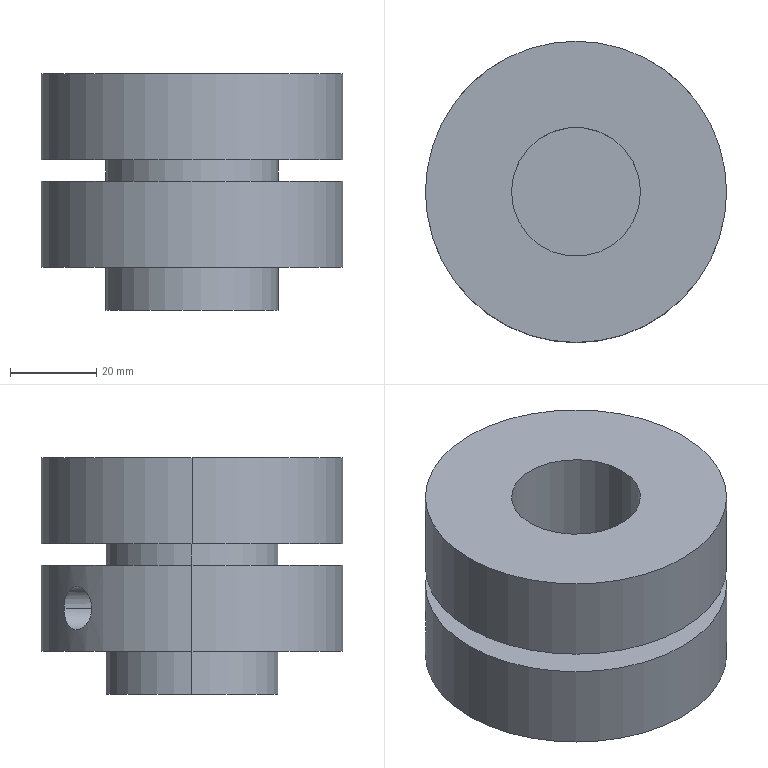Part | SolidWorks | features ICE 3, RevCut 2, Extrusion 1 | 1 solid | 22 faces | box 70 x 70 x 55 mm | volume 152574 mm3 | cylinder 14 | plane 8 | commonest cylinder face diameters 10 x4 40 x4 70 x4 30 x2
STEP:
#1=CARTESIAN_POINT('',(18.437,29.75,-15.));
#2=VERTEX_POINT('',#1);
#3=CARTESIAN_POINT('',(26.097,23.323,-15.));
#4=VERTEX_POINT('',#3);
#5=CARTESIAN_POINT('',(18.437,29.75,-15.));
#6=CARTESIAN_POINT('',(18.437,29.75,-15.326));
#7=CARTESIAN_POINT('',(18.464,29.734,-15.651));
#8=CARTESIAN_POINT('',(18.574,29.665,-16.297));
#9=CARTESIAN_POINT('',(18.656,29.614,-16.612));
#10=CARTESIAN_POINT('',(18.868,29.479,-17.214));
#11=CARTESIAN_POINT('',(19.,29.394,-17.505));
#12=CARTESIAN_POINT('',(19.308,29.193,-18.051));
#13=CARTESIAN_POINT('',(19.481,29.078,-18.303));
#14=CARTESIAN_POINT('',(19.864,28.818,-18.764));
#15=CARTESIAN_POINT('',(20.076,28.671,-18.975));
#16=CARTESIAN_POINT('',(20.519,28.356,-19.338));
#17=CARTESIAN_POINT('',(20.751,28.186,-19.491));
#18=CARTESIAN_POINT('',(21.115,27.914,-19.68));
#19=CARTESIAN_POINT('',(21.24,27.819,-19.736));
#20=CARTESIAN_POINT('',(21.489,27.627,-19.832));
#21=CARTESIAN_POINT('',(21.613,27.53,-19.871));
#22=CARTESIAN_POINT('',(21.989,27.232,-19.967));
#23=CARTESIAN_POINT('',(22.242,27.026,-20.));
#24=CARTESIAN_POINT('',(22.748,26.601,-20.));
#25=CARTESIAN_POINT('',(22.994,26.389,-19.968));
#26=CARTESIAN_POINT('',(23.473,25.964,-19.841));
#27=CARTESIAN_POINT('',(23.708,25.749,-19.745));
#28=CARTESIAN_POINT('',(24.15,25.335,-19.494));
#29=CARTESIAN_POINT('',(24.358,25.135,-19.341));
#30=CARTESIAN_POINT('',(24.746,24.753,-18.979));
#31=CARTESIAN_POINT('',(24.928,24.57,-18.768));
#32=CARTESIAN_POINT('',(25.251,24.238,-18.308));
#33=CARTESIAN_POINT('',(25.394,24.087,-18.057));
#34=CARTESIAN_POINT('',(25.647,23.818,-17.51));
#35=CARTESIAN_POINT('',(25.753,23.703,-17.22));
#36=CARTESIAN_POINT('',(25.923,23.517,-16.619));
#37=CARTESIAN_POINT('',(25.988,23.444,-16.304));
#38=CARTESIAN_POINT('',(26.075,23.347,-15.658));
#39=CARTESIAN_POINT('',(26.097,23.323,-15.331));
#40=CARTESIAN_POINT('',(26.097,23.323,-15.));
#41=B_SPLINE_CURVE_WITH_KNOTS('',3,(#5,#6,#7,#8,#9,#10,#11,#12,#13,#14,#15,#16,#17,#18,#19,#20,#21,#22,#23,#24,#25,#26,#27,#28,#29,#30,#31,#32,#33,#34,#35,#36,#37,#38,#39,#40),.UNSPECIFIED.,.F.,.F.,(4,2,2,2,2,2,2,2,2,2,2,2,2,2,2,2,2,4),(0.01565,0.01663,0.01761,0.01859,0.01956,0.02054,0.02152,0.02201,0.0225,0.02348,0.02445,0.02543,0.02641,0.02739,0.02837,0.02934,0.03032,0.0313),.UNSPECIFIED.);
#42=EDGE_CURVE('',#2,#4,#41,.T.);
#43=ORIENTED_EDGE('',*,*,#42,.F.);
#44=CARTESIAN_POINT('',(8.621,18.052,-15.));
#45=VERTEX_POINT('',#44);
#46=CARTESIAN_POINT('',(8.621,18.052,-15.));
#47=DIRECTION('',(-0.6428,-0.766,0.));
#48=VECTOR('',#47,1000.);
#49=LINE('',#46,#48);
#50=EDGE_CURVE('',#2,#45,#49,.T.);
#51=ORIENTED_EDGE('',*,*,#50,.T.);
#52=CARTESIAN_POINT('',(16.281,11.624,-15.));
#53=VERTEX_POINT('',#52);
#54=CARTESIAN_POINT('',(12.451,14.838,-15.));
#55=DIRECTION('',(-0.6428,-0.766,0.));
#56=DIRECTION('',(0.766,-0.6428,0.));
#57=AXIS2_PLACEMENT_3D('',#54,#55,#56);
#58=CIRCLE('',#57,5.);
#59=EDGE_CURVE('',#45,#53,#58,.T.);
#60=ORIENTED_EDGE('',*,*,#59,.T.);
#61=CARTESIAN_POINT('',(16.281,11.624,-15.));
#62=DIRECTION('',(-0.6428,-0.766,0.));
#63=VECTOR('',#62,1000.);
#64=LINE('',#61,#63);
#65=EDGE_CURVE('',#4,#53,#64,.T.);
#66=ORIENTED_EDGE('',*,*,#65,.F.);
#67=EDGE_LOOP('',(#43,#51,#60,#66));
#68=FACE_OUTER_BOUND('',#67,.T.);
#69=CARTESIAN_POINT('',(12.451,14.838,-15.));
#70=DIRECTION('',(-0.6428,-0.766,0.));
#71=DIRECTION('',(0.766,-0.6428,0.));
#72=AXIS2_PLACEMENT_3D('',#69,#70,#71);
#73=CYLINDRICAL_SURFACE('',#72,5.);
#74=ADVANCED_FACE('',(#68),#73,.F.);
#75=CARTESIAN_POINT('',(-26.097,23.323,-15.));
#76=VERTEX_POINT('',#75);
#77=CARTESIAN_POINT('',(-18.437,29.75,-15.));
#78=VERTEX_POINT('',#77);
#79=CARTESIAN_POINT('',(-26.097,23.323,-15.));
#80=CARTESIAN_POINT('',(-26.097,23.323,-15.326));
#81=CARTESIAN_POINT('',(-26.076,23.347,-15.651));
#82=CARTESIAN_POINT('',(-25.989,23.443,-16.297));
#83=CARTESIAN_POINT('',(-25.924,23.515,-16.612));
#84=CARTESIAN_POINT('',(-25.755,23.7,-17.214));
#85=CARTESIAN_POINT('',(-25.649,23.816,-17.505));
#86=CARTESIAN_POINT('',(-25.397,24.084,-18.051));
#87=CARTESIAN_POINT('',(-25.254,24.234,-18.303));
#88=CARTESIAN_POINT('',(-24.931,24.566,-18.764));
#89=CARTESIAN_POINT('',(-24.75,24.749,-18.975));
#90=CARTESIAN_POINT('',(-24.362,25.131,-19.338));
#91=CARTESIAN_POINT('',(-24.155,25.331,-19.491));
#92=CARTESIAN_POINT('',(-23.823,25.642,-19.68));
#93=CARTESIAN_POINT('',(-23.708,25.748,-19.736));
#94=CARTESIAN_POINT('',(-23.476,25.959,-19.832));
#95=CARTESIAN_POINT('',(-23.358,26.066,-19.871));
#96=CARTESIAN_POINT('',(-23.,26.384,-19.967));
#97=CARTESIAN_POINT('',(-22.753,26.597,-20.));
#98=CARTESIAN_POINT('',(-22.247,27.022,-20.));
#99=CARTESIAN_POINT('',(-21.995,27.227,-19.968));
#100=CARTESIAN_POINT('',(-21.493,27.625,-19.841));
#101=CARTESIAN_POINT('',(-21.241,27.819,-19.745));
#102=CARTESIAN_POINT('',(-20.756,28.183,-19.494));
#103=CARTESIAN_POINT('',(-20.524,28.352,-19.341));
#104=CARTESIAN_POINT('',(-20.08,28.669,-18.979));
#105=CARTESIAN_POINT('',(-19.868,28.815,-18.768));
#106=CARTESIAN_POINT('',(-19.485,29.076,-18.308));
#107=CARTESIAN_POINT('',(-19.311,29.191,-18.057));
#108=CARTESIAN_POINT('',(-19.002,29.393,-17.51));
#109=CARTESIAN_POINT('',(-18.871,29.477,-17.22));
#110=CARTESIAN_POINT('',(-18.658,29.612,-16.619));
#111=CARTESIAN_POINT('',(-18.575,29.664,-16.304));
#112=CARTESIAN_POINT('',(-18.465,29.733,-15.658));
#113=CARTESIAN_POINT('',(-18.437,29.75,-15.331));
#114=CARTESIAN_POINT('',(-18.437,29.75,-15.));
#115=B_SPLINE_CURVE_WITH_KNOTS('',3,(#79,#80,#81,#82,#83,#84,#85,#86,#87,#88,#89,#90,#91,#92,#93,#94,#95,#96,#97,#98,#99,#100,#101,#102,#103,#104,#105,#106,#107,#108,#109,#110,#111,#112,#113,#114),.UNSPECIFIED.,.F.,.F.,(4,2,2,2,2,2,2,2,2,2,2,2,2,2,2,2,2,4),(0.01565,0.01663,0.01761,0.01859,0.01956,0.02054,0.02152,0.02201,0.0225,0.02348,0.02445,0.02543,0.02641,0.02739,0.02837,0.02934,0.03032,0.0313),.UNSPECIFIED.);
#116=EDGE_CURVE('',#76,#78,#115,.T.);
#117=ORIENTED_EDGE('',*,*,#116,.F.);
#118=CARTESIAN_POINT('',(-15.454,10.638,-15.));
#119=VERTEX_POINT('',#118);
#120=CARTESIAN_POINT('',(-15.454,10.638,-15.));
#121=DIRECTION('',(0.6428,-0.766,0.));
#122=VECTOR('',#121,1000.);
#123=LINE('',#120,#122);
#124=EDGE_CURVE('',#76,#119,#123,.T.);
#125=ORIENTED_EDGE('',*,*,#124,.T.);
#126=CARTESIAN_POINT('',(-7.793,17.066,-15.));
#127=VERTEX_POINT('',#126);
#128=CARTESIAN_POINT('',(-11.623,13.852,-15.));
#129=DIRECTION('',(0.6428,-0.766,0.));
#130=DIRECTION('',(0.766,0.6428,0.));
#131=AXIS2_PLACEMENT_3D('',#128,#129,#130);
#132=CIRCLE('',#131,5.);
#133=EDGE_CURVE('',#119,#127,#132,.T.);
#134=ORIENTED_EDGE('',*,*,#133,.T.);
#135=CARTESIAN_POINT('',(-7.793,17.066,-15.));
#136=DIRECTION('',(0.6428,-0.766,0.));
#137=VECTOR('',#136,1000.);
#138=LINE('',#135,#137);
#139=EDGE_CURVE('',#78,#127,#138,.T.);
#140=ORIENTED_EDGE('',*,*,#139,.F.);
#141=EDGE_LOOP('',(#117,#125,#134,#140));
#142=FACE_OUTER_BOUND('',#141,.T.);
#143=CARTESIAN_POINT('',(-11.623,13.852,-15.));
#144=DIRECTION('',(0.6428,-0.766,0.));
#145=DIRECTION('',(0.766,0.6428,0.));
#146=AXIS2_PLACEMENT_3D('',#143,#144,#145);
#147=CYLINDRICAL_SURFACE('',#146,5.);
#148=ADVANCED_FACE('',(#142),#147,.F.);
#149=CARTESIAN_POINT('',(-20.,0.,-35.));
#150=VERTEX_POINT('',#149);
#151=CARTESIAN_POINT('',(20.,0.,-35.));
#152=VERTEX_POINT('',#151);
#153=CARTESIAN_POINT('',(0.,0.,-35.));
#154=DIRECTION('',(0.,0.,-1.));
#155=DIRECTION('',(-1.,0.,0.));
#156=AXIS2_PLACEMENT_3D('',#153,#154,#155);
#157=CIRCLE('',#156,20.);
#158=EDGE_CURVE('',#150,#152,#157,.T.);
#159=ORIENTED_EDGE('',*,*,#158,.F.);
#160=CARTESIAN_POINT('',(-20.,0.,-25.));
#161=VERTEX_POINT('',#160);
#162=CARTESIAN_POINT('',(-20.,0.,-35.));
#163=DIRECTION('',(0.,0.,1.));
#164=VECTOR('',#163,1000.);
#165=LINE('',#162,#164);
#166=EDGE_CURVE('',#150,#161,#165,.T.);
#167=ORIENTED_EDGE('',*,*,#166,.T.);
#168=CARTESIAN_POINT('',(20.,0.,-25.));
#169=VERTEX_POINT('',#168);
#170=CARTESIAN_POINT('',(0.,0.,-25.));
#171=DIRECTION('',(0.,0.,-1.));
#172=DIRECTION('',(-1.,0.,0.));
#173=AXIS2_PLACEMENT_3D('',#170,#171,#172);
#174=CIRCLE('',#173,20.);
#175=EDGE_CURVE('',#161,#169,#174,.T.);
#176=ORIENTED_EDGE('',*,*,#175,.T.);
#177=CARTESIAN_POINT('',(20.,0.,-35.));
#178=DIRECTION('',(0.,0.,1.));
#179=VECTOR('',#178,1000.);
#180=LINE('',#177,#179);
#181=EDGE_CURVE('',#152,#169,#180,.T.);
#182=ORIENTED_EDGE('',*,*,#181,.F.);
#183=EDGE_LOOP('',(#159,#167,#176,#182));
#184=FACE_OUTER_BOUND('',#183,.T.);
#185=CARTESIAN_POINT('',(0.,0.,-35.));
#186=DIRECTION('',(0.,0.,1.));
#187=DIRECTION('',(1.,0.,0.));
#188=AXIS2_PLACEMENT_3D('',#185,#186,#187);
#189=CYLINDRICAL_SURFACE('',#188,20.);
#190=ADVANCED_FACE('',(#184),#189,.T.);
#191=CARTESIAN_POINT('',(26.097,23.323,-15.));
#192=CARTESIAN_POINT('',(26.097,23.323,-14.669));
#193=CARTESIAN_POINT('',(26.075,23.347,-14.344));
#194=CARTESIAN_POINT('',(26.011,23.419,-13.864));
#195=CARTESIAN_POINT('',(25.984,23.449,-13.706));
#196=CARTESIAN_POINT('',(25.919,23.52,-13.391));
#197=CARTESIAN_POINT('',(25.881,23.562,-13.235));
#198=CARTESIAN_POINT('',(25.753,23.702,-12.781));
#199=CARTESIAN_POINT('',(25.648,23.816,-12.494));
#200=CARTESIAN_POINT('',(25.398,24.083,-11.951));
#201=CARTESIAN_POINT('',(25.252,24.236,-11.694));
#202=CARTESIAN_POINT('',(24.929,24.568,-11.233));
#203=CARTESIAN_POINT('',(24.751,24.748,-11.027));
#204=CARTESIAN_POINT('',(24.361,25.132,-10.661));
#205=CARTESIAN_POINT('',(24.151,25.334,-10.506));
#206=CARTESIAN_POINT('',(23.711,25.746,-10.257));
#207=CARTESIAN_POINT('',(23.478,25.959,-10.16));
#208=CARTESIAN_POINT('',(22.995,26.388,-10.032));
#209=CARTESIAN_POINT('',(22.749,26.6,-10.));
#210=CARTESIAN_POINT('',(22.249,27.02,-10.));
#211=CARTESIAN_POINT('',(21.992,27.23,-10.033));
#212=CARTESIAN_POINT('',(21.489,27.629,-10.16));
#213=CARTESIAN_POINT('',(21.241,27.819,-10.255));
#214=CARTESIAN_POINT('',(20.877,28.092,-10.443));
#215=CARTESIAN_POINT('',(20.756,28.181,-10.514));
#216=CARTESIAN_POINT('',(20.522,28.352,-10.669));
#217=CARTESIAN_POINT('',(20.408,28.434,-10.753));
#218=CARTESIAN_POINT('',(20.077,28.671,-11.024));
#219=CARTESIAN_POINT('',(19.868,28.815,-11.231));
#220=CARTESIAN_POINT('',(19.481,29.079,-11.697));
#221=CARTESIAN_POINT('',(19.307,29.193,-11.949));
#222=CARTESIAN_POINT('',(19.002,29.393,-12.491));
#223=CARTESIAN_POINT('',(18.869,29.478,-12.783));
#224=CARTESIAN_POINT('',(18.656,29.614,-13.388));
#225=CARTESIAN_POINT('',(18.575,29.665,-13.7));
#226=CARTESIAN_POINT('',(18.465,29.733,-14.342));
#227=CARTESIAN_POINT('',(18.437,29.75,-14.673));
#228=CARTESIAN_POINT('',(18.437,29.75,-15.));
#229=B_SPLINE_CURVE_WITH_KNOTS('',3,(#191,#192,#193,#194,#195,#196,#197,#198,#199,#200,#201,#202,#203,#204,#205,#206,#207,#208,#209,#210,#211,#212,#213,#214,#215,#216,#217,#218,#219,#220,#221,#222,#223,#224,#225,#226,#227,#228),.UNSPECIFIED.,.F.,.F.,(4,2,2,2,2,2,2,2,2,2,2,2,2,2,2,2,2,2,4),(0.,0.0009783,0.001467,0.001957,0.002935,0.003913,0.004891,0.00587,0.006848,0.007826,0.008804,0.009783,0.01027,0.01076,0.01174,0.01272,0.0137,0.01467,0.01565),.UNSPECIFIED.);
#230=EDGE_CURVE('',#4,#2,#229,.T.);
#231=ORIENTED_EDGE('',*,*,#230,.T.);
#232=ORIENTED_EDGE('',*,*,#42,.T.);
#233=EDGE_LOOP('',(#231,#232));
#234=FACE_BOUND('',#233,.T.);
#235=CARTESIAN_POINT('',(-18.437,29.75,-15.));
#236=CARTESIAN_POINT('',(-18.437,29.75,-14.669));
#237=CARTESIAN_POINT('',(-18.465,29.733,-14.344));
#238=CARTESIAN_POINT('',(-18.546,29.682,-13.864));
#239=CARTESIAN_POINT('',(-18.58,29.661,-13.706));
#240=CARTESIAN_POINT('',(-18.662,29.61,-13.391));
#241=CARTESIAN_POINT('',(-18.71,29.58,-13.235));
#242=CARTESIAN_POINT('',(-18.87,29.478,-12.781));
#243=CARTESIAN_POINT('',(-19.,29.394,-12.494));
#244=CARTESIAN_POINT('',(-19.306,29.194,-11.951));
#245=CARTESIAN_POINT('',(-19.483,29.077,-11.694));
#246=CARTESIAN_POINT('',(-19.866,28.816,-11.233));
#247=CARTESIAN_POINT('',(-20.074,28.673,-11.027));
#248=CARTESIAN_POINT('',(-20.52,28.355,-10.661));
#249=CARTESIAN_POINT('',(-20.756,28.183,-10.506));
#250=CARTESIAN_POINT('',(-21.238,27.822,-10.257));
#251=CARTESIAN_POINT('',(-21.488,27.629,-10.16));
#252=CARTESIAN_POINT('',(-21.994,27.228,-10.032));
#253=CARTESIAN_POINT('',(-22.246,27.023,-10.));
#254=CARTESIAN_POINT('',(-22.746,26.603,-10.));
#255=CARTESIAN_POINT('',(-22.997,26.386,-10.033));
#256=CARTESIAN_POINT('',(-23.477,25.96,-10.16));
#257=CARTESIAN_POINT('',(-23.708,25.749,-10.255));
#258=CARTESIAN_POINT('',(-24.04,25.438,-10.443));
#259=CARTESIAN_POINT('',(-24.149,25.335,-10.514));
#260=CARTESIAN_POINT('',(-24.358,25.134,-10.669));
#261=CARTESIAN_POINT('',(-24.458,25.036,-10.753));
#262=CARTESIAN_POINT('',(-24.749,24.75,-11.024));
#263=CARTESIAN_POINT('',(-24.927,24.57,-11.231));
#264=CARTESIAN_POINT('',(-25.254,24.234,-11.697));
#265=CARTESIAN_POINT('',(-25.397,24.083,-11.949));
#266=CARTESIAN_POINT('',(-25.647,23.818,-12.491));
#267=CARTESIAN_POINT('',(-25.754,23.701,-12.783));
#268=CARTESIAN_POINT('',(-25.925,23.515,-13.388));
#269=CARTESIAN_POINT('',(-25.989,23.444,-13.7));
#270=CARTESIAN_POINT('',(-26.075,23.347,-14.342));
#271=CARTESIAN_POINT('',(-26.097,23.323,-14.673));
#272=CARTESIAN_POINT('',(-26.097,23.323,-15.));
#273=B_SPLINE_CURVE_WITH_KNOTS('',3,(#235,#236,#237,#238,#239,#240,#241,#242,#243,#244,#245,#246,#247,#248,#249,#250,#251,#252,#253,#254,#255,#256,#257,#258,#259,#260,#261,#262,#263,#264,#265,#266,#267,#268,#269,#270,#271,#272),.UNSPECIFIED.,.F.,.F.,(4,2,2,2,2,2,2,2,2,2,2,2,2,2,2,2,2,2,4),(0.,0.0009783,0.001467,0.001957,0.002935,0.003913,0.004891,0.00587,0.006848,0.007826,0.008804,0.009783,0.01027,0.01076,0.01174,0.01272,0.0137,0.01467,0.01565),.UNSPECIFIED.);
#274=EDGE_CURVE('',#78,#76,#273,.T.);
#275=ORIENTED_EDGE('',*,*,#274,.T.);
#276=ORIENTED_EDGE('',*,*,#116,.T.);
#277=EDGE_LOOP('',(#275,#276));
#278=FACE_BOUND('',#277,.T.);
#279=CARTESIAN_POINT('',(-35.,0.,-25.));
#280=VERTEX_POINT('',#279);
#281=CARTESIAN_POINT('',(35.,0.,-25.));
#282=VERTEX_POINT('',#281);
#283=CARTESIAN_POINT('',(0.,0.,-25.));
#284=DIRECTION('',(0.,0.,-1.));
#285=DIRECTION('',(-1.,0.,0.));
#286=AXIS2_PLACEMENT_3D('',#283,#284,#285);
#287=CIRCLE('',#286,35.);
#288=EDGE_CURVE('',#280,#282,#287,.T.);
#289=ORIENTED_EDGE('',*,*,#288,.F.);
#290=CARTESIAN_POINT('',(-35.,0.,-5.));
#291=VERTEX_POINT('',#290);
#292=CARTESIAN_POINT('',(-35.,0.,-25.));
#293=DIRECTION('',(0.,0.,1.));
#294=VECTOR('',#293,1000.);
#295=LINE('',#292,#294);
#296=EDGE_CURVE('',#280,#291,#295,.T.);
#297=ORIENTED_EDGE('',*,*,#296,.T.);
#298=CARTESIAN_POINT('',(35.,0.,-5.));
#299=VERTEX_POINT('',#298);
#300=CARTESIAN_POINT('',(0.,0.,-5.));
#301=DIRECTION('',(0.,0.,-1.));
#302=DIRECTION('',(-1.,0.,0.));
#303=AXIS2_PLACEMENT_3D('',#300,#301,#302);
#304=CIRCLE('',#303,35.);
#305=EDGE_CURVE('',#291,#299,#304,.T.);
#306=ORIENTED_EDGE('',*,*,#305,.T.);
#307=CARTESIAN_POINT('',(35.,0.,-25.));
#308=DIRECTION('',(0.,0.,1.));
#309=VECTOR('',#308,1000.);
#310=LINE('',#307,#309);
#311=EDGE_CURVE('',#282,#299,#310,.T.);
#312=ORIENTED_EDGE('',*,*,#311,.F.);
#313=EDGE_LOOP('',(#289,#297,#306,#312));
#314=FACE_OUTER_BOUND('',#313,.T.);
#315=CARTESIAN_POINT('',(0.,0.,-25.));
#316=DIRECTION('',(0.,0.,1.));
#317=DIRECTION('',(1.,0.,0.));
#318=AXIS2_PLACEMENT_3D('',#315,#316,#317);
#319=CYLINDRICAL_SURFACE('',#318,35.);
#320=ADVANCED_FACE('',(#234,#278,#314),#319,.T.);
#321=CARTESIAN_POINT('',(-20.,0.,-5.));
#322=VERTEX_POINT('',#321);
#323=CARTESIAN_POINT('',(20.,0.,-5.));
#324=VERTEX_POINT('',#323);
#325=CARTESIAN_POINT('',(0.,0.,-5.));
#326=DIRECTION('',(0.,0.,-1.));
#327=DIRECTION('',(-1.,0.,0.));
#328=AXIS2_PLACEMENT_3D('',#325,#326,#327);
#329=CIRCLE('',#328,20.);
#330=EDGE_CURVE('',#322,#324,#329,.T.);
#331=ORIENTED_EDGE('',*,*,#330,.F.);
#332=CARTESIAN_POINT('',(-20.,0.,0.));
#333=VERTEX_POINT('',#332);
#334=CARTESIAN_POINT('',(-20.,0.,-5.));
#335=DIRECTION('',(0.,0.,1.));
#336=VECTOR('',#335,1000.);
#337=LINE('',#334,#336);
#338=EDGE_CURVE('',#322,#333,#337,.T.);
#339=ORIENTED_EDGE('',*,*,#338,.T.);
#340=CARTESIAN_POINT('',(20.,0.,0.));
#341=VERTEX_POINT('',#340);
#342=CARTESIAN_POINT('',(0.,0.,0.));
#343=DIRECTION('',(0.,0.,-1.));
#344=DIRECTION('',(1.,0.,0.));
#345=AXIS2_PLACEMENT_3D('',#342,#343,#344);
#346=CIRCLE('',#345,20.);
#347=EDGE_CURVE('',#333,#341,#346,.T.);
#348=ORIENTED_EDGE('',*,*,#347,.T.);
#349=CARTESIAN_POINT('',(20.,0.,-5.));
#350=DIRECTION('',(0.,0.,1.));
#351=VECTOR('',#350,1000.);
#352=LINE('',#349,#351);
#353=EDGE_CURVE('',#324,#341,#352,.T.);
#354=ORIENTED_EDGE('',*,*,#353,.F.);
#355=EDGE_LOOP('',(#331,#339,#348,#354));
#356=FACE_OUTER_BOUND('',#355,.T.);
#357=CARTESIAN_POINT('',(0.,0.,-5.));
#358=DIRECTION('',(0.,0.,1.));
#359=DIRECTION('',(1.,0.,0.));
#360=AXIS2_PLACEMENT_3D('',#357,#358,#359);
#361=CYLINDRICAL_SURFACE('',#360,20.);
#362=ADVANCED_FACE('',(#356),#361,.T.);
#363=CARTESIAN_POINT('',(-15.,0.,20.));
#364=VERTEX_POINT('',#363);
#365=CARTESIAN_POINT('',(15.,0.,20.));
#366=VERTEX_POINT('',#365);
#367=CARTESIAN_POINT('',(0.,0.,20.));
#368=DIRECTION('',(0.,0.,1.));
#369=DIRECTION('',(1.,0.,0.));
#370=AXIS2_PLACEMENT_3D('',#367,#368,#369);
#371=CIRCLE('',#370,15.);
#372=EDGE_CURVE('',#364,#366,#371,.T.);
#373=ORIENTED_EDGE('',*,*,#372,.T.);
#374=CARTESIAN_POINT('',(15.,0.,-5.));
#375=VERTEX_POINT('',#374);
#376=CARTESIAN_POINT('',(15.,0.,20.));
#377=DIRECTION('',(0.,0.,-1.));
#378=VECTOR('',#377,1000.);
#379=LINE('',#376,#378);
#380=EDGE_CURVE('',#366,#375,#379,.T.);
#381=ORIENTED_EDGE('',*,*,#380,.T.);
#382=CARTESIAN_POINT('',(-15.,0.,-5.));
#383=VERTEX_POINT('',#382);
#384=CARTESIAN_POINT('',(0.,0.,-5.));
#385=DIRECTION('',(0.,0.,1.));
#386=DIRECTION('',(-1.,0.,0.));
#387=AXIS2_PLACEMENT_3D('',#384,#385,#386);
#388=CIRCLE('',#387,15.);
#389=EDGE_CURVE('',#383,#375,#388,.T.);
#390=ORIENTED_EDGE('',*,*,#389,.F.);
#391=CARTESIAN_POINT('',(-15.,0.,20.));
#392=DIRECTION('',(0.,0.,-1.));
#393=VECTOR('',#392,1000.);
#394=LINE('',#391,#393);
#395=EDGE_CURVE('',#364,#383,#394,.T.);
#396=ORIENTED_EDGE('',*,*,#395,.F.);
#397=EDGE_LOOP('',(#373,#381,#390,#396));
#398=FACE_OUTER_BOUND('',#397,.T.);
#399=CARTESIAN_POINT('',(0.,0.,20.));
#400=DIRECTION('',(0.,0.,-1.));
#401=DIRECTION('',(-1.,0.,0.));
#402=AXIS2_PLACEMENT_3D('',#399,#400,#401);
#403=CYLINDRICAL_SURFACE('',#402,15.);
#404=ADVANCED_FACE('',(#398),#403,.F.);
#405=CARTESIAN_POINT('',(35.,0.,20.));
#406=VERTEX_POINT('',#405);
#407=CARTESIAN_POINT('',(-35.,0.,20.));
#408=VERTEX_POINT('',#407);
#409=CARTESIAN_POINT('',(0.,0.,20.));
#410=DIRECTION('',(0.,0.,1.));
#411=DIRECTION('',(1.,0.,0.));
#412=AXIS2_PLACEMENT_3D('',#409,#410,#411);
#413=CIRCLE('',#412,35.);
#414=EDGE_CURVE('',#406,#408,#413,.T.);
#415=ORIENTED_EDGE('',*,*,#414,.F.);
#416=CARTESIAN_POINT('',(35.,0.,0.));
#417=VERTEX_POINT('',#416);
#418=CARTESIAN_POINT('',(35.,0.,20.));
#419=DIRECTION('',(0.,0.,-1.));
#420=VECTOR('',#419,1000.);
#421=LINE('',#418,#420);
#422=EDGE_CURVE('',#406,#417,#421,.T.);
#423=ORIENTED_EDGE('',*,*,#422,.T.);
#424=CARTESIAN_POINT('',(-35.,0.,0.));
#425=VERTEX_POINT('',#424);
#426=CARTESIAN_POINT('',(0.,0.,0.));
#427=DIRECTION('',(0.,0.,1.));
#428=DIRECTION('',(1.,0.,0.));
#429=AXIS2_PLACEMENT_3D('',#426,#427,#428);
#430=CIRCLE('',#429,35.);
#431=EDGE_CURVE('',#417,#425,#430,.T.);
#432=ORIENTED_EDGE('',*,*,#431,.T.);
#433=CARTESIAN_POINT('',(-35.,0.,20.));
#434=DIRECTION('',(0.,0.,-1.));
#435=VECTOR('',#434,1000.);
#436=LINE('',#433,#435);
#437=EDGE_CURVE('',#408,#425,#436,.T.);
#438=ORIENTED_EDGE('',*,*,#437,.F.);
#439=EDGE_LOOP('',(#415,#423,#432,#438));
#440=FACE_OUTER_BOUND('',#439,.T.);
#441=CARTESIAN_POINT('',(0.,0.,20.));
#442=DIRECTION('',(0.,0.,-1.));
#443=DIRECTION('',(-1.,0.,0.));
#444=AXIS2_PLACEMENT_3D('',#441,#442,#443);
#445=CYLINDRICAL_SURFACE('',#444,35.);
#446=ADVANCED_FACE('',(#440),#445,.T.);
#447=CARTESIAN_POINT('',(0.,0.,20.));
#448=DIRECTION('',(0.,0.,1.));
#449=DIRECTION('',(1.,0.,0.));
#450=AXIS2_PLACEMENT_3D('',#447,#448,#449);
#451=CIRCLE('',#450,35.);
#452=EDGE_CURVE('',#408,#406,#451,.T.);
#453=ORIENTED_EDGE('',*,*,#452,.T.);
#454=ORIENTED_EDGE('',*,*,#414,.T.);
#455=EDGE_LOOP('',(#453,#454));
#456=FACE_OUTER_BOUND('',#455,.T.);
#457=ORIENTED_EDGE('',*,*,#372,.F.);
#458=CARTESIAN_POINT('',(0.,0.,20.));
#459=DIRECTION('',(0.,0.,1.));
#460=DIRECTION('',(1.,0.,0.));
#461=AXIS2_PLACEMENT_3D('',#458,#459,#460);
#462=CIRCLE('',#461,15.);
#463=EDGE_CURVE('',#366,#364,#462,.T.);
#464=ORIENTED_EDGE('',*,*,#463,.F.);
#465=EDGE_LOOP('',(#457,#464));
#466=FACE_BOUND('',#465,.T.);
#467=CARTESIAN_POINT('',(0.,0.,20.));
#468=DIRECTION('',(0.,0.,1.));
#469=DIRECTION('',(1.,0.,0.));
#470=AXIS2_PLACEMENT_3D('',#467,#468,#469);
#471=PLANE('',#470);
#472=ADVANCED_FACE('',(#456,#466),#471,.T.);
#473=CARTESIAN_POINT('',(0.,0.,0.));
#474=DIRECTION('',(0.,0.,-1.));
#475=DIRECTION('',(1.,0.,0.));
#476=AXIS2_PLACEMENT_3D('',#473,#474,#475);
#477=CIRCLE('',#476,20.);
#478=EDGE_CURVE('',#341,#333,#477,.T.);
#479=ORIENTED_EDGE('',*,*,#478,.F.);
#480=ORIENTED_EDGE('',*,*,#347,.F.);
#481=EDGE_LOOP('',(#479,#480));
#482=FACE_BOUND('',#481,.T.);
#483=CARTESIAN_POINT('',(0.,0.,0.));
#484=DIRECTION('',(0.,0.,1.));
#485=DIRECTION('',(1.,0.,0.));
#486=AXIS2_PLACEMENT_3D('',#483,#484,#485);
#487=CIRCLE('',#486,35.);
#488=EDGE_CURVE('',#425,#417,#487,.T.);
#489=ORIENTED_EDGE('',*,*,#488,.F.);
#490=ORIENTED_EDGE('',*,*,#431,.F.);
#491=EDGE_LOOP('',(#489,#490));
#492=FACE_OUTER_BOUND('',#491,.T.);
#493=CARTESIAN_POINT('',(0.,0.,0.));
#494=DIRECTION('',(0.,0.,1.));
#495=DIRECTION('',(1.,0.,0.));
#496=AXIS2_PLACEMENT_3D('',#493,#494,#495);
#497=PLANE('',#496);
#498=ADVANCED_FACE('',(#482,#492),#497,.F.);
#499=ORIENTED_EDGE('',*,*,#422,.F.);
#500=ORIENTED_EDGE('',*,*,#452,.F.);
#501=ORIENTED_EDGE('',*,*,#437,.T.);
#502=ORIENTED_EDGE('',*,*,#488,.T.);
#503=EDGE_LOOP('',(#499,#500,#501,#502));
#504=FACE_OUTER_BOUND('',#503,.T.);
#505=CARTESIAN_POINT('',(0.,0.,20.));
#506=DIRECTION('',(0.,0.,-1.));
#507=DIRECTION('',(-1.,0.,0.));
#508=AXIS2_PLACEMENT_3D('',#505,#506,#507);
#509=CYLINDRICAL_SURFACE('',#508,35.);
#510=ADVANCED_FACE('',(#504),#509,.T.);
#511=ORIENTED_EDGE('',*,*,#380,.F.);
#512=ORIENTED_EDGE('',*,*,#463,.T.);
#513=ORIENTED_EDGE('',*,*,#395,.T.);
#514=CARTESIAN_POINT('',(0.,0.,-5.));
#515=DIRECTION('',(0.,0.,1.));
#516=DIRECTION('',(-1.,0.,0.));
#517=AXIS2_PLACEMENT_3D('',#514,#515,#516);
#518=CIRCLE('',#517,15.);
#519=EDGE_CURVE('',#375,#383,#518,.T.);
#520=ORIENTED_EDGE('',*,*,#519,.F.);
#521=EDGE_LOOP('',(#511,#512,#513,#520));
#522=FACE_OUTER_BOUND('',#521,.T.);
#523=CARTESIAN_POINT('',(0.,0.,20.));
#524=DIRECTION('',(0.,0.,-1.));
#525=DIRECTION('',(-1.,0.,0.));
#526=AXIS2_PLACEMENT_3D('',#523,#524,#525);
#527=CYLINDRICAL_SURFACE('',#526,15.);
#528=ADVANCED_FACE('',(#522),#527,.F.);
#529=ORIENTED_EDGE('',*,*,#338,.F.);
#530=CARTESIAN_POINT('',(0.,0.,-5.));
#531=DIRECTION('',(0.,0.,-1.));
#532=DIRECTION('',(-1.,0.,0.));
#533=AXIS2_PLACEMENT_3D('',#530,#531,#532);
#534=CIRCLE('',#533,20.);
#535=EDGE_CURVE('',#324,#322,#534,.T.);
#536=ORIENTED_EDGE('',*,*,#535,.F.);
#537=ORIENTED_EDGE('',*,*,#353,.T.);
#538=ORIENTED_EDGE('',*,*,#478,.T.);
#539=EDGE_LOOP('',(#529,#536,#537,#538));
#540=FACE_OUTER_BOUND('',#539,.T.);
#541=CARTESIAN_POINT('',(0.,0.,-5.));
#542=DIRECTION('',(0.,0.,1.));
#543=DIRECTION('',(1.,0.,0.));
#544=AXIS2_PLACEMENT_3D('',#541,#542,#543);
#545=CYLINDRICAL_SURFACE('',#544,20.);
#546=ADVANCED_FACE('',(#540),#545,.T.);
#547=ORIENTED_EDGE('',*,*,#535,.T.);
#548=ORIENTED_EDGE('',*,*,#330,.T.);
#549=EDGE_LOOP('',(#547,#548));
#550=FACE_BOUND('',#549,.T.);
#551=CARTESIAN_POINT('',(0.,0.,-5.));
#552=DIRECTION('',(0.,0.,-1.));
#553=DIRECTION('',(-1.,0.,0.));
#554=AXIS2_PLACEMENT_3D('',#551,#552,#553);
#555=CIRCLE('',#554,35.);
#556=EDGE_CURVE('',#299,#291,#555,.T.);
#557=ORIENTED_EDGE('',*,*,#556,.F.);
#558=ORIENTED_EDGE('',*,*,#305,.F.);
#559=EDGE_LOOP('',(#557,#558));
#560=FACE_OUTER_BOUND('',#559,.T.);
#561=CARTESIAN_POINT('',(0.,0.,-5.));
#562=DIRECTION('',(0.,0.,-1.));
#563=DIRECTION('',(-1.,0.,0.));
#564=AXIS2_PLACEMENT_3D('',#561,#562,#563);
#565=PLANE('',#564);
#566=ADVANCED_FACE('',(#550,#560),#565,.F.);
#567=CARTESIAN_POINT('',(0.,0.,-25.));
#568=DIRECTION('',(0.,0.,-1.));
#569=DIRECTION('',(-1.,0.,0.));
#570=AXIS2_PLACEMENT_3D('',#567,#568,#569);
#571=CIRCLE('',#570,20.);
#572=EDGE_CURVE('',#169,#161,#571,.T.);
#573=ORIENTED_EDGE('',*,*,#572,.F.);
#574=ORIENTED_EDGE('',*,*,#175,.F.);
#575=EDGE_LOOP('',(#573,#574));
#576=FACE_BOUND('',#575,.T.);
#577=CARTESIAN_POINT('',(0.,0.,-25.));
#578=DIRECTION('',(0.,0.,-1.));
#579=DIRECTION('',(-1.,0.,0.));
#580=AXIS2_PLACEMENT_3D('',#577,#578,#579);
#581=CIRCLE('',#580,35.);
#582=EDGE_CURVE('',#282,#280,#581,.T.);
#583=ORIENTED_EDGE('',*,*,#582,.T.);
#584=ORIENTED_EDGE('',*,*,#288,.T.);
#585=EDGE_LOOP('',(#583,#584));
#586=FACE_OUTER_BOUND('',#585,.T.);
#587=CARTESIAN_POINT('',(0.,0.,-25.));
#588=DIRECTION('',(0.,0.,-1.));
#589=DIRECTION('',(-1.,0.,0.));
#590=AXIS2_PLACEMENT_3D('',#587,#588,#589);
#591=PLANE('',#590);
#592=ADVANCED_FACE('',(#576,#586),#591,.T.);
#593=ORIENTED_EDGE('',*,*,#296,.F.);
#594=ORIENTED_EDGE('',*,*,#582,.F.);
#595=ORIENTED_EDGE('',*,*,#311,.T.);
#596=ORIENTED_EDGE('',*,*,#556,.T.);
#597=EDGE_LOOP('',(#593,#594,#595,#596));
#598=FACE_OUTER_BOUND('',#597,.T.);
#599=CARTESIAN_POINT('',(0.,0.,-25.));
#600=DIRECTION('',(0.,0.,1.));
#601=DIRECTION('',(1.,0.,0.));
#602=AXIS2_PLACEMENT_3D('',#599,#600,#601);
#603=CYLINDRICAL_SURFACE('',#602,35.);
#604=ADVANCED_FACE('',(#598),#603,.T.);
#605=ORIENTED_EDGE('',*,*,#389,.T.);
#606=ORIENTED_EDGE('',*,*,#519,.T.);
#607=EDGE_LOOP('',(#605,#606));
#608=FACE_OUTER_BOUND('',#607,.T.);
#609=CARTESIAN_POINT('',(0.,0.,-5.));
#610=DIRECTION('',(0.,0.,-1.));
#611=DIRECTION('',(-1.,0.,0.));
#612=AXIS2_PLACEMENT_3D('',#609,#610,#611);
#613=PLANE('',#612);
#614=ADVANCED_FACE('',(#608),#613,.F.);
#615=ORIENTED_EDGE('',*,*,#166,.F.);
#616=CARTESIAN_POINT('',(0.,0.,-35.));
#617=DIRECTION('',(0.,0.,-1.));
#618=DIRECTION('',(-1.,0.,0.));
#619=AXIS2_PLACEMENT_3D('',#616,#617,#618);
#620=CIRCLE('',#619,20.);
#621=EDGE_CURVE('',#152,#150,#620,.T.);
#622=ORIENTED_EDGE('',*,*,#621,.F.);
#623=ORIENTED_EDGE('',*,*,#181,.T.);
#624=ORIENTED_EDGE('',*,*,#572,.T.);
#625=EDGE_LOOP('',(#615,#622,#623,#624));
#626=FACE_OUTER_BOUND('',#625,.T.);
#627=CARTESIAN_POINT('',(0.,0.,-35.));
#628=DIRECTION('',(0.,0.,1.));
#629=DIRECTION('',(1.,0.,0.));
#630=AXIS2_PLACEMENT_3D('',#627,#628,#629);
#631=CYLINDRICAL_SURFACE('',#630,20.);
#632=ADVANCED_FACE('',(#626),#631,.T.);
#633=ORIENTED_EDGE('',*,*,#621,.T.);
#634=ORIENTED_EDGE('',*,*,#158,.T.);
#635=EDGE_LOOP('',(#633,#634));
#636=FACE_OUTER_BOUND('',#635,.T.);
#637=CARTESIAN_POINT('',(0.,0.,-35.));
#638=DIRECTION('',(0.,0.,-1.));
#639=DIRECTION('',(-1.,0.,0.));
#640=AXIS2_PLACEMENT_3D('',#637,#638,#639);
#641=PLANE('',#640);
#642=ADVANCED_FACE('',(#636),#641,.T.);
#643=ORIENTED_EDGE('',*,*,#124,.F.);
#644=ORIENTED_EDGE('',*,*,#274,.F.);
#645=ORIENTED_EDGE('',*,*,#139,.T.);
#646=CARTESIAN_POINT('',(-11.623,13.852,-15.));
#647=DIRECTION('',(0.6428,-0.766,0.));
#648=DIRECTION('',(0.766,0.6428,0.));
#649=AXIS2_PLACEMENT_3D('',#646,#647,#648);
#650=CIRCLE('',#649,5.);
#651=EDGE_CURVE('',#127,#119,#650,.T.);
#652=ORIENTED_EDGE('',*,*,#651,.T.);
#653=EDGE_LOOP('',(#643,#644,#645,#652));
#654=FACE_OUTER_BOUND('',#653,.T.);
#655=CARTESIAN_POINT('',(-11.623,13.852,-15.));
#656=DIRECTION('',(0.6428,-0.766,0.));
#657=DIRECTION('',(0.766,0.6428,0.));
#658=AXIS2_PLACEMENT_3D('',#655,#656,#657);
#659=CYLINDRICAL_SURFACE('',#658,5.);
#660=ADVANCED_FACE('',(#654),#659,.F.);
#661=ORIENTED_EDGE('',*,*,#651,.F.);
#662=ORIENTED_EDGE('',*,*,#133,.F.);
#663=EDGE_LOOP('',(#661,#662));
#664=FACE_OUTER_BOUND('',#663,.T.);
#665=CARTESIAN_POINT('',(-7.793,17.066,-15.));
#666=DIRECTION('',(0.6428,-0.766,0.));
#667=DIRECTION('',(0.766,0.6428,0.));
#668=AXIS2_PLACEMENT_3D('',#665,#666,#667);
#669=PLANE('',#668);
#670=ADVANCED_FACE('',(#664),#669,.F.);
#671=ORIENTED_EDGE('',*,*,#50,.F.);
#672=ORIENTED_EDGE('',*,*,#230,.F.);
#673=ORIENTED_EDGE('',*,*,#65,.T.);
#674=CARTESIAN_POINT('',(12.451,14.838,-15.));
#675=DIRECTION('',(-0.6428,-0.766,0.));
#676=DIRECTION('',(0.766,-0.6428,0.));
#677=AXIS2_PLACEMENT_3D('',#674,#675,#676);
#678=CIRCLE('',#677,5.);
#679=EDGE_CURVE('',#53,#45,#678,.T.);
#680=ORIENTED_EDGE('',*,*,#679,.T.);
#681=EDGE_LOOP('',(#671,#672,#673,#680));
#682=FACE_OUTER_BOUND('',#681,.T.);
#683=CARTESIAN_POINT('',(12.451,14.838,-15.));
#684=DIRECTION('',(-0.6428,-0.766,0.));
#685=DIRECTION('',(0.766,-0.6428,0.));
#686=AXIS2_PLACEMENT_3D('',#683,#684,#685);
#687=CYLINDRICAL_SURFACE('',#686,5.);
#688=ADVANCED_FACE('',(#682),#687,.F.);
#689=ORIENTED_EDGE('',*,*,#679,.F.);
#690=ORIENTED_EDGE('',*,*,#59,.F.);
#691=EDGE_LOOP('',(#689,#690));
#692=FACE_OUTER_BOUND('',#691,.T.);
#693=CARTESIAN_POINT('',(16.281,11.624,-15.));
#694=DIRECTION('',(-0.6428,-0.766,0.));
#695=DIRECTION('',(0.766,-0.6428,0.));
#696=AXIS2_PLACEMENT_3D('',#693,#694,#695);
#697=PLANE('',#696);
#698=ADVANCED_FACE('',(#692),#697,.F.);
#699=CLOSED_SHELL('',(#74,#148,#190,#320,#362,#404,#446,#472,#498,#510,#528,#546,#566,#592,#604,#614,#632,#642,#660,#670,#688,#698));
#700=MANIFOLD_SOLID_BREP('',#699);
#701=CARTESIAN_POINT('',(0.,0.,0.));
#702=DIRECTION('',(0.,0.,1.));
#703=DIRECTION('',(1.,0.,0.));
#704=AXIS2_PLACEMENT_3D('',#701,#702,#703);
#705=(LENGTH_UNIT()NAMED_UNIT(*)SI_UNIT(.MILLI.,.METRE.));
#706=UNCERTAINTY_MEASURE_WITH_UNIT(LENGTH_MEASURE(0.00001),#705,'','');
#707=(NAMED_UNIT(*)PLANE_ANGLE_UNIT()SI_UNIT($,.RADIAN.));
#708=(NAMED_UNIT(*)SI_UNIT($,.STERADIAN.)SOLID_ANGLE_UNIT());
#709=(GEOMETRIC_REPRESENTATION_CONTEXT(3)GLOBAL_UNCERTAINTY_ASSIGNED_CONTEXT((#706))GLOBAL_UNIT_ASSIGNED_CONTEXT((#705,#707,#708))REPRESENTATION_CONTEXT('',''));
#710=ADVANCED_BREP_SHAPE_REPRESENTATION('',(#700,#704),#709);